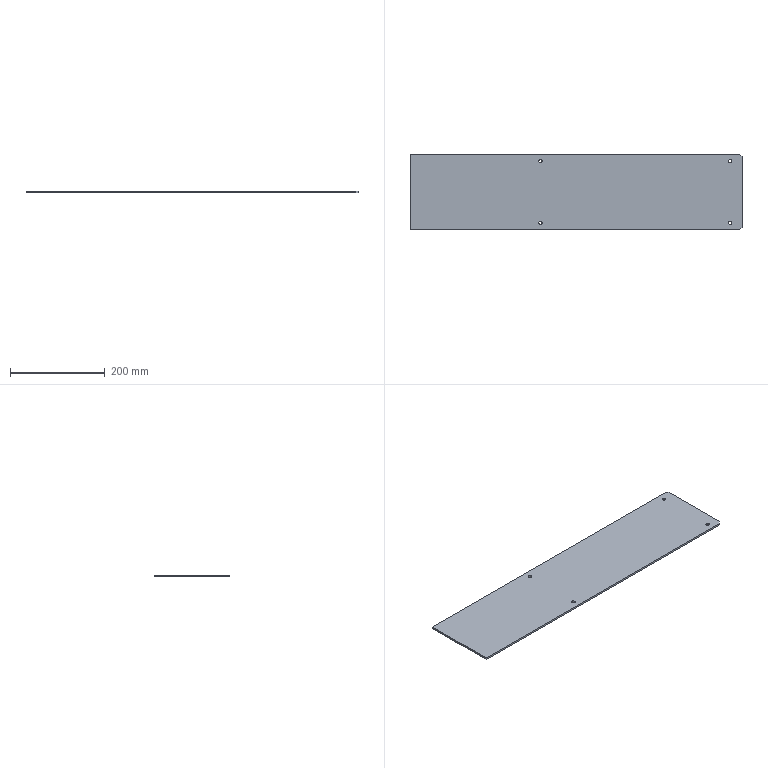Part | SolidWorks | features Chamfer 1, Extrusion 1, ICE 1 | 1 solid | 16 faces | box 700 x 160 x 4 mm | volume 447284 mm3 | cylinder 8 | plane 8 | commonest cylinder face diameters 7 x8
STEP:
#1=CARTESIAN_POINT('',(-78.5,-65.,0.));
#2=VERTEX_POINT('',#1);
#3=CARTESIAN_POINT('',(-71.5,-65.,0.));
#4=VERTEX_POINT('',#3);
#5=CARTESIAN_POINT('',(-75.,-65.,0.));
#6=DIRECTION('',(0.,0.,1.));
#7=DIRECTION('',(1.,0.,0.));
#8=AXIS2_PLACEMENT_3D('',#5,#6,#7);
#9=CIRCLE('',#8,3.5);
#10=EDGE_CURVE('',#2,#4,#9,.T.);
#11=ORIENTED_EDGE('',*,*,#10,.F.);
#12=CARTESIAN_POINT('',(-78.5,-65.,4.));
#13=VERTEX_POINT('',#12);
#14=CARTESIAN_POINT('',(-78.5,-65.,0.));
#15=DIRECTION('',(0.,0.,1.));
#16=VECTOR('',#15,1000.);
#17=LINE('',#14,#16);
#18=EDGE_CURVE('',#2,#13,#17,.T.);
#19=ORIENTED_EDGE('',*,*,#18,.T.);
#20=CARTESIAN_POINT('',(-71.5,-65.,4.));
#21=VERTEX_POINT('',#20);
#22=CARTESIAN_POINT('',(-75.,-65.,4.));
#23=DIRECTION('',(0.,0.,1.));
#24=DIRECTION('',(1.,0.,0.));
#25=AXIS2_PLACEMENT_3D('',#22,#23,#24);
#26=CIRCLE('',#25,3.5);
#27=EDGE_CURVE('',#13,#21,#26,.T.);
#28=ORIENTED_EDGE('',*,*,#27,.T.);
#29=CARTESIAN_POINT('',(-71.5,-65.,0.));
#30=DIRECTION('',(0.,0.,1.));
#31=VECTOR('',#30,1000.);
#32=LINE('',#29,#31);
#33=EDGE_CURVE('',#4,#21,#32,.T.);
#34=ORIENTED_EDGE('',*,*,#33,.F.);
#35=EDGE_LOOP('',(#11,#19,#28,#34));
#36=FACE_OUTER_BOUND('',#35,.T.);
#37=CARTESIAN_POINT('',(-75.,-65.,0.));
#38=DIRECTION('',(0.,0.,1.));
#39=DIRECTION('',(1.,0.,0.));
#40=AXIS2_PLACEMENT_3D('',#37,#38,#39);
#41=CYLINDRICAL_SURFACE('',#40,3.5);
#42=ADVANCED_FACE('',(#36),#41,.F.);
#43=CARTESIAN_POINT('',(321.5,-65.,0.));
#44=VERTEX_POINT('',#43);
#45=CARTESIAN_POINT('',(328.5,-65.,0.));
#46=VERTEX_POINT('',#45);
#47=CARTESIAN_POINT('',(325.,-65.,0.));
#48=DIRECTION('',(0.,0.,1.));
#49=DIRECTION('',(1.,0.,0.));
#50=AXIS2_PLACEMENT_3D('',#47,#48,#49);
#51=CIRCLE('',#50,3.5);
#52=EDGE_CURVE('',#44,#46,#51,.T.);
#53=ORIENTED_EDGE('',*,*,#52,.F.);
#54=CARTESIAN_POINT('',(321.5,-65.,4.));
#55=VERTEX_POINT('',#54);
#56=CARTESIAN_POINT('',(321.5,-65.,0.));
#57=DIRECTION('',(0.,0.,1.));
#58=VECTOR('',#57,1000.);
#59=LINE('',#56,#58);
#60=EDGE_CURVE('',#44,#55,#59,.T.);
#61=ORIENTED_EDGE('',*,*,#60,.T.);
#62=CARTESIAN_POINT('',(328.5,-65.,4.));
#63=VERTEX_POINT('',#62);
#64=CARTESIAN_POINT('',(325.,-65.,4.));
#65=DIRECTION('',(0.,0.,1.));
#66=DIRECTION('',(1.,0.,0.));
#67=AXIS2_PLACEMENT_3D('',#64,#65,#66);
#68=CIRCLE('',#67,3.5);
#69=EDGE_CURVE('',#55,#63,#68,.T.);
#70=ORIENTED_EDGE('',*,*,#69,.T.);
#71=CARTESIAN_POINT('',(328.5,-65.,0.));
#72=DIRECTION('',(0.,0.,1.));
#73=VECTOR('',#72,1000.);
#74=LINE('',#71,#73);
#75=EDGE_CURVE('',#46,#63,#74,.T.);
#76=ORIENTED_EDGE('',*,*,#75,.F.);
#77=EDGE_LOOP('',(#53,#61,#70,#76));
#78=FACE_OUTER_BOUND('',#77,.T.);
#79=CARTESIAN_POINT('',(325.,-65.,0.));
#80=DIRECTION('',(0.,0.,1.));
#81=DIRECTION('',(1.,0.,0.));
#82=AXIS2_PLACEMENT_3D('',#79,#80,#81);
#83=CYLINDRICAL_SURFACE('',#82,3.5);
#84=ADVANCED_FACE('',(#78),#83,.F.);
#85=CARTESIAN_POINT('',(321.5,65.,0.));
#86=VERTEX_POINT('',#85);
#87=CARTESIAN_POINT('',(328.5,65.,0.));
#88=VERTEX_POINT('',#87);
#89=CARTESIAN_POINT('',(325.,65.,0.));
#90=DIRECTION('',(0.,0.,1.));
#91=DIRECTION('',(1.,0.,0.));
#92=AXIS2_PLACEMENT_3D('',#89,#90,#91);
#93=CIRCLE('',#92,3.5);
#94=EDGE_CURVE('',#86,#88,#93,.T.);
#95=ORIENTED_EDGE('',*,*,#94,.F.);
#96=CARTESIAN_POINT('',(321.5,65.,4.));
#97=VERTEX_POINT('',#96);
#98=CARTESIAN_POINT('',(321.5,65.,0.));
#99=DIRECTION('',(0.,0.,1.));
#100=VECTOR('',#99,1000.);
#101=LINE('',#98,#100);
#102=EDGE_CURVE('',#86,#97,#101,.T.);
#103=ORIENTED_EDGE('',*,*,#102,.T.);
#104=CARTESIAN_POINT('',(328.5,65.,4.));
#105=VERTEX_POINT('',#104);
#106=CARTESIAN_POINT('',(325.,65.,4.));
#107=DIRECTION('',(0.,0.,1.));
#108=DIRECTION('',(1.,0.,0.));
#109=AXIS2_PLACEMENT_3D('',#106,#107,#108);
#110=CIRCLE('',#109,3.5);
#111=EDGE_CURVE('',#97,#105,#110,.T.);
#112=ORIENTED_EDGE('',*,*,#111,.T.);
#113=CARTESIAN_POINT('',(328.5,65.,0.));
#114=DIRECTION('',(0.,0.,1.));
#115=VECTOR('',#114,1000.);
#116=LINE('',#113,#115);
#117=EDGE_CURVE('',#88,#105,#116,.T.);
#118=ORIENTED_EDGE('',*,*,#117,.F.);
#119=EDGE_LOOP('',(#95,#103,#112,#118));
#120=FACE_OUTER_BOUND('',#119,.T.);
#121=CARTESIAN_POINT('',(325.,65.,0.));
#122=DIRECTION('',(0.,0.,1.));
#123=DIRECTION('',(1.,0.,0.));
#124=AXIS2_PLACEMENT_3D('',#121,#122,#123);
#125=CYLINDRICAL_SURFACE('',#124,3.5);
#126=ADVANCED_FACE('',(#120),#125,.F.);
#127=CARTESIAN_POINT('',(-78.5,65.,0.));
#128=VERTEX_POINT('',#127);
#129=CARTESIAN_POINT('',(-71.5,65.,0.));
#130=VERTEX_POINT('',#129);
#131=CARTESIAN_POINT('',(-75.,65.,0.));
#132=DIRECTION('',(0.,0.,1.));
#133=DIRECTION('',(1.,0.,0.));
#134=AXIS2_PLACEMENT_3D('',#131,#132,#133);
#135=CIRCLE('',#134,3.5);
#136=EDGE_CURVE('',#128,#130,#135,.T.);
#137=ORIENTED_EDGE('',*,*,#136,.F.);
#138=CARTESIAN_POINT('',(-78.5,65.,4.));
#139=VERTEX_POINT('',#138);
#140=CARTESIAN_POINT('',(-78.5,65.,0.));
#141=DIRECTION('',(0.,0.,1.));
#142=VECTOR('',#141,1000.);
#143=LINE('',#140,#142);
#144=EDGE_CURVE('',#128,#139,#143,.T.);
#145=ORIENTED_EDGE('',*,*,#144,.T.);
#146=CARTESIAN_POINT('',(-71.5,65.,4.));
#147=VERTEX_POINT('',#146);
#148=CARTESIAN_POINT('',(-75.,65.,4.));
#149=DIRECTION('',(0.,0.,1.));
#150=DIRECTION('',(1.,0.,0.));
#151=AXIS2_PLACEMENT_3D('',#148,#149,#150);
#152=CIRCLE('',#151,3.5);
#153=EDGE_CURVE('',#139,#147,#152,.T.);
#154=ORIENTED_EDGE('',*,*,#153,.T.);
#155=CARTESIAN_POINT('',(-71.5,65.,0.));
#156=DIRECTION('',(0.,0.,1.));
#157=VECTOR('',#156,1000.);
#158=LINE('',#155,#157);
#159=EDGE_CURVE('',#130,#147,#158,.T.);
#160=ORIENTED_EDGE('',*,*,#159,.F.);
#161=EDGE_LOOP('',(#137,#145,#154,#160));
#162=FACE_OUTER_BOUND('',#161,.T.);
#163=CARTESIAN_POINT('',(-75.,65.,0.));
#164=DIRECTION('',(0.,0.,1.));
#165=DIRECTION('',(1.,0.,0.));
#166=AXIS2_PLACEMENT_3D('',#163,#164,#165);
#167=CYLINDRICAL_SURFACE('',#166,3.5);
#168=ADVANCED_FACE('',(#162),#167,.F.);
#169=CARTESIAN_POINT('',(-350.,-80.,0.));
#170=VERTEX_POINT('',#169);
#171=CARTESIAN_POINT('',(345.,-80.,0.));
#172=VERTEX_POINT('',#171);
#173=CARTESIAN_POINT('',(-350.,-80.,0.));
#174=DIRECTION('',(1.,0.,0.));
#175=VECTOR('',#174,1000.);
#176=LINE('',#173,#175);
#177=EDGE_CURVE('',#170,#172,#176,.T.);
#178=ORIENTED_EDGE('',*,*,#177,.T.);
#179=CARTESIAN_POINT('',(345.,-80.,4.));
#180=VERTEX_POINT('',#179);
#181=CARTESIAN_POINT('',(345.,-80.,4.));
#182=DIRECTION('',(0.,0.,1.));
#183=VECTOR('',#182,1000.);
#184=LINE('',#181,#183);
#185=EDGE_CURVE('',#172,#180,#184,.T.);
#186=ORIENTED_EDGE('',*,*,#185,.T.);
#187=CARTESIAN_POINT('',(-350.,-80.,4.));
#188=VERTEX_POINT('',#187);
#189=CARTESIAN_POINT('',(-350.,-80.,4.));
#190=DIRECTION('',(1.,0.,0.));
#191=VECTOR('',#190,1000.);
#192=LINE('',#189,#191);
#193=EDGE_CURVE('',#188,#180,#192,.T.);
#194=ORIENTED_EDGE('',*,*,#193,.F.);
#195=CARTESIAN_POINT('',(-350.,-80.,4.));
#196=DIRECTION('',(0.,0.,-1.));
#197=VECTOR('',#196,1000.);
#198=LINE('',#195,#197);
#199=EDGE_CURVE('',#188,#170,#198,.T.);
#200=ORIENTED_EDGE('',*,*,#199,.T.);
#201=EDGE_LOOP('',(#178,#186,#194,#200));
#202=FACE_OUTER_BOUND('',#201,.T.);
#203=CARTESIAN_POINT('',(-350.,-80.,4.));
#204=DIRECTION('',(0.,1.,0.));
#205=DIRECTION('',(0.,0.,1.));
#206=AXIS2_PLACEMENT_3D('',#203,#204,#205);
#207=PLANE('',#206);
#208=ADVANCED_FACE('',(#202),#207,.F.);
#209=CARTESIAN_POINT('',(350.,75.,4.));
#210=VERTEX_POINT('',#209);
#211=CARTESIAN_POINT('',(350.,-75.,4.));
#212=VERTEX_POINT('',#211);
#213=CARTESIAN_POINT('',(350.,80.,4.));
#214=DIRECTION('',(0.,-1.,0.));
#215=VECTOR('',#214,1000.);
#216=LINE('',#213,#215);
#217=EDGE_CURVE('',#210,#212,#216,.T.);
#218=ORIENTED_EDGE('',*,*,#217,.T.);
#219=CARTESIAN_POINT('',(350.,-75.,0.));
#220=VERTEX_POINT('',#219);
#221=CARTESIAN_POINT('',(350.,-75.,0.));
#222=DIRECTION('',(0.,0.,-1.));
#223=VECTOR('',#222,1000.);
#224=LINE('',#221,#223);
#225=EDGE_CURVE('',#212,#220,#224,.T.);
#226=ORIENTED_EDGE('',*,*,#225,.T.);
#227=CARTESIAN_POINT('',(350.,75.,0.));
#228=VERTEX_POINT('',#227);
#229=CARTESIAN_POINT('',(350.,80.,0.));
#230=DIRECTION('',(0.,-1.,0.));
#231=VECTOR('',#230,1000.);
#232=LINE('',#229,#231);
#233=EDGE_CURVE('',#228,#220,#232,.T.);
#234=ORIENTED_EDGE('',*,*,#233,.F.);
#235=CARTESIAN_POINT('',(350.,75.,4.));
#236=DIRECTION('',(0.,0.,1.));
#237=VECTOR('',#236,1000.);
#238=LINE('',#235,#237);
#239=EDGE_CURVE('',#228,#210,#238,.T.);
#240=ORIENTED_EDGE('',*,*,#239,.T.);
#241=EDGE_LOOP('',(#218,#226,#234,#240));
#242=FACE_OUTER_BOUND('',#241,.T.);
#243=CARTESIAN_POINT('',(350.,80.,4.));
#244=DIRECTION('',(1.,0.,0.));
#245=DIRECTION('',(0.,0.,-1.));
#246=AXIS2_PLACEMENT_3D('',#243,#244,#245);
#247=PLANE('',#246);
#248=ADVANCED_FACE('',(#242),#247,.T.);
#249=CARTESIAN_POINT('',(-350.,80.,4.));
#250=VERTEX_POINT('',#249);
#251=CARTESIAN_POINT('',(345.,80.,4.));
#252=VERTEX_POINT('',#251);
#253=CARTESIAN_POINT('',(-350.,80.,4.));
#254=DIRECTION('',(1.,0.,0.));
#255=VECTOR('',#254,1000.);
#256=LINE('',#253,#255);
#257=EDGE_CURVE('',#250,#252,#256,.T.);
#258=ORIENTED_EDGE('',*,*,#257,.T.);
#259=CARTESIAN_POINT('',(345.,80.,0.));
#260=VERTEX_POINT('',#259);
#261=CARTESIAN_POINT('',(345.,80.,4.));
#262=DIRECTION('',(0.,0.,-1.));
#263=VECTOR('',#262,1000.);
#264=LINE('',#261,#263);
#265=EDGE_CURVE('',#252,#260,#264,.T.);
#266=ORIENTED_EDGE('',*,*,#265,.T.);
#267=CARTESIAN_POINT('',(-350.,80.,0.));
#268=VERTEX_POINT('',#267);
#269=CARTESIAN_POINT('',(-350.,80.,0.));
#270=DIRECTION('',(1.,0.,0.));
#271=VECTOR('',#270,1000.);
#272=LINE('',#269,#271);
#273=EDGE_CURVE('',#268,#260,#272,.T.);
#274=ORIENTED_EDGE('',*,*,#273,.F.);
#275=CARTESIAN_POINT('',(-350.,80.,4.));
#276=DIRECTION('',(0.,0.,-1.));
#277=VECTOR('',#276,1000.);
#278=LINE('',#275,#277);
#279=EDGE_CURVE('',#250,#268,#278,.T.);
#280=ORIENTED_EDGE('',*,*,#279,.F.);
#281=EDGE_LOOP('',(#258,#266,#274,#280));
#282=FACE_OUTER_BOUND('',#281,.T.);
#283=CARTESIAN_POINT('',(-350.,80.,4.));
#284=DIRECTION('',(0.,1.,0.));
#285=DIRECTION('',(0.,0.,1.));
#286=AXIS2_PLACEMENT_3D('',#283,#284,#285);
#287=PLANE('',#286);
#288=ADVANCED_FACE('',(#282),#287,.T.);
#289=CARTESIAN_POINT('',(-350.,80.,0.));
#290=DIRECTION('',(0.,-1.,0.));
#291=VECTOR('',#290,1000.);
#292=LINE('',#289,#291);
#293=EDGE_CURVE('',#268,#170,#292,.T.);
#294=ORIENTED_EDGE('',*,*,#293,.T.);
#295=ORIENTED_EDGE('',*,*,#199,.F.);
#296=CARTESIAN_POINT('',(-350.,80.,4.));
#297=DIRECTION('',(0.,-1.,0.));
#298=VECTOR('',#297,1000.);
#299=LINE('',#296,#298);
#300=EDGE_CURVE('',#250,#188,#299,.T.);
#301=ORIENTED_EDGE('',*,*,#300,.F.);
#302=ORIENTED_EDGE('',*,*,#279,.T.);
#303=EDGE_LOOP('',(#294,#295,#301,#302));
#304=FACE_OUTER_BOUND('',#303,.T.);
#305=CARTESIAN_POINT('',(-350.,80.,4.));
#306=DIRECTION('',(1.,0.,0.));
#307=DIRECTION('',(0.,1.,0.));
#308=AXIS2_PLACEMENT_3D('',#305,#306,#307);
#309=PLANE('',#308);
#310=ADVANCED_FACE('',(#304),#309,.F.);
#311=CARTESIAN_POINT('',(-75.,-65.,4.));
#312=DIRECTION('',(0.,0.,1.));
#313=DIRECTION('',(1.,0.,0.));
#314=AXIS2_PLACEMENT_3D('',#311,#312,#313);
#315=CIRCLE('',#314,3.5);
#316=EDGE_CURVE('',#21,#13,#315,.T.);
#317=ORIENTED_EDGE('',*,*,#316,.F.);
#318=ORIENTED_EDGE('',*,*,#27,.F.);
#319=EDGE_LOOP('',(#317,#318));
#320=FACE_BOUND('',#319,.T.);
#321=CARTESIAN_POINT('',(325.,-65.,4.));
#322=DIRECTION('',(0.,0.,1.));
#323=DIRECTION('',(1.,0.,0.));
#324=AXIS2_PLACEMENT_3D('',#321,#322,#323);
#325=CIRCLE('',#324,3.5);
#326=EDGE_CURVE('',#63,#55,#325,.T.);
#327=ORIENTED_EDGE('',*,*,#326,.F.);
#328=ORIENTED_EDGE('',*,*,#69,.F.);
#329=EDGE_LOOP('',(#327,#328));
#330=FACE_BOUND('',#329,.T.);
#331=CARTESIAN_POINT('',(325.,65.,4.));
#332=DIRECTION('',(0.,0.,1.));
#333=DIRECTION('',(1.,0.,0.));
#334=AXIS2_PLACEMENT_3D('',#331,#332,#333);
#335=CIRCLE('',#334,3.5);
#336=EDGE_CURVE('',#105,#97,#335,.T.);
#337=ORIENTED_EDGE('',*,*,#336,.F.);
#338=ORIENTED_EDGE('',*,*,#111,.F.);
#339=EDGE_LOOP('',(#337,#338));
#340=FACE_BOUND('',#339,.T.);
#341=CARTESIAN_POINT('',(-75.,65.,4.));
#342=DIRECTION('',(0.,0.,1.));
#343=DIRECTION('',(1.,0.,0.));
#344=AXIS2_PLACEMENT_3D('',#341,#342,#343);
#345=CIRCLE('',#344,3.5);
#346=EDGE_CURVE('',#147,#139,#345,.T.);
#347=ORIENTED_EDGE('',*,*,#346,.F.);
#348=ORIENTED_EDGE('',*,*,#153,.F.);
#349=EDGE_LOOP('',(#347,#348));
#350=FACE_BOUND('',#349,.T.);
#351=ORIENTED_EDGE('',*,*,#193,.T.);
#352=CARTESIAN_POINT('',(350.,-75.,4.));
#353=DIRECTION('',(0.7071,0.7071,0.));
#354=VECTOR('',#353,1000.);
#355=LINE('',#352,#354);
#356=EDGE_CURVE('',#180,#212,#355,.T.);
#357=ORIENTED_EDGE('',*,*,#356,.T.);
#358=ORIENTED_EDGE('',*,*,#217,.F.);
#359=CARTESIAN_POINT('',(345.,80.,4.));
#360=DIRECTION('',(-0.7071,0.7071,0.));
#361=VECTOR('',#360,1000.);
#362=LINE('',#359,#361);
#363=EDGE_CURVE('',#210,#252,#362,.T.);
#364=ORIENTED_EDGE('',*,*,#363,.T.);
#365=ORIENTED_EDGE('',*,*,#257,.F.);
#366=ORIENTED_EDGE('',*,*,#300,.T.);
#367=EDGE_LOOP('',(#351,#357,#358,#364,#365,#366));
#368=FACE_OUTER_BOUND('',#367,.T.);
#369=CARTESIAN_POINT('',(0.,0.,4.));
#370=DIRECTION('',(0.,0.,-1.));
#371=DIRECTION('',(-1.,0.,0.));
#372=AXIS2_PLACEMENT_3D('',#369,#370,#371);
#373=PLANE('',#372);
#374=ADVANCED_FACE('',(#320,#330,#340,#350,#368),#373,.F.);
#375=CARTESIAN_POINT('',(-75.,-65.,0.));
#376=DIRECTION('',(0.,0.,1.));
#377=DIRECTION('',(1.,0.,0.));
#378=AXIS2_PLACEMENT_3D('',#375,#376,#377);
#379=CIRCLE('',#378,3.5);
#380=EDGE_CURVE('',#4,#2,#379,.T.);
#381=ORIENTED_EDGE('',*,*,#380,.T.);
#382=ORIENTED_EDGE('',*,*,#10,.T.);
#383=EDGE_LOOP('',(#381,#382));
#384=FACE_BOUND('',#383,.T.);
#385=CARTESIAN_POINT('',(325.,-65.,0.));
#386=DIRECTION('',(0.,0.,1.));
#387=DIRECTION('',(1.,0.,0.));
#388=AXIS2_PLACEMENT_3D('',#385,#386,#387);
#389=CIRCLE('',#388,3.5);
#390=EDGE_CURVE('',#46,#44,#389,.T.);
#391=ORIENTED_EDGE('',*,*,#390,.T.);
#392=ORIENTED_EDGE('',*,*,#52,.T.);
#393=EDGE_LOOP('',(#391,#392));
#394=FACE_BOUND('',#393,.T.);
#395=CARTESIAN_POINT('',(325.,65.,0.));
#396=DIRECTION('',(0.,0.,1.));
#397=DIRECTION('',(1.,0.,0.));
#398=AXIS2_PLACEMENT_3D('',#395,#396,#397);
#399=CIRCLE('',#398,3.5);
#400=EDGE_CURVE('',#88,#86,#399,.T.);
#401=ORIENTED_EDGE('',*,*,#400,.T.);
#402=ORIENTED_EDGE('',*,*,#94,.T.);
#403=EDGE_LOOP('',(#401,#402));
#404=FACE_BOUND('',#403,.T.);
#405=CARTESIAN_POINT('',(-75.,65.,0.));
#406=DIRECTION('',(0.,0.,1.));
#407=DIRECTION('',(1.,0.,0.));
#408=AXIS2_PLACEMENT_3D('',#405,#406,#407);
#409=CIRCLE('',#408,3.5);
#410=EDGE_CURVE('',#130,#128,#409,.T.);
#411=ORIENTED_EDGE('',*,*,#410,.T.);
#412=ORIENTED_EDGE('',*,*,#136,.T.);
#413=EDGE_LOOP('',(#411,#412));
#414=FACE_BOUND('',#413,.T.);
#415=ORIENTED_EDGE('',*,*,#233,.T.);
#416=CARTESIAN_POINT('',(212.5,-212.5,0.));
#417=DIRECTION('',(-0.7071,-0.7071,0.));
#418=VECTOR('',#417,1000.);
#419=LINE('',#416,#418);
#420=EDGE_CURVE('',#220,#172,#419,.T.);
#421=ORIENTED_EDGE('',*,*,#420,.T.);
#422=ORIENTED_EDGE('',*,*,#177,.F.);
#423=ORIENTED_EDGE('',*,*,#293,.F.);
#424=ORIENTED_EDGE('',*,*,#273,.T.);
#425=CARTESIAN_POINT('',(212.5,212.5,0.));
#426=DIRECTION('',(0.7071,-0.7071,0.));
#427=VECTOR('',#426,1000.);
#428=LINE('',#425,#427);
#429=EDGE_CURVE('',#260,#228,#428,.T.);
#430=ORIENTED_EDGE('',*,*,#429,.T.);
#431=EDGE_LOOP('',(#415,#421,#422,#423,#424,#430));
#432=FACE_OUTER_BOUND('',#431,.T.);
#433=CARTESIAN_POINT('',(0.,0.,0.));
#434=DIRECTION('',(0.,0.,-1.));
#435=DIRECTION('',(-1.,0.,0.));
#436=AXIS2_PLACEMENT_3D('',#433,#434,#435);
#437=PLANE('',#436);
#438=ADVANCED_FACE('',(#384,#394,#404,#414,#432),#437,.T.);
#439=ORIENTED_EDGE('',*,*,#144,.F.);
#440=ORIENTED_EDGE('',*,*,#410,.F.);
#441=ORIENTED_EDGE('',*,*,#159,.T.);
#442=ORIENTED_EDGE('',*,*,#346,.T.);
#443=EDGE_LOOP('',(#439,#440,#441,#442));
#444=FACE_OUTER_BOUND('',#443,.T.);
#445=CARTESIAN_POINT('',(-75.,65.,0.));
#446=DIRECTION('',(0.,0.,1.));
#447=DIRECTION('',(1.,0.,0.));
#448=AXIS2_PLACEMENT_3D('',#445,#446,#447);
#449=CYLINDRICAL_SURFACE('',#448,3.5);
#450=ADVANCED_FACE('',(#444),#449,.F.);
#451=ORIENTED_EDGE('',*,*,#102,.F.);
#452=ORIENTED_EDGE('',*,*,#400,.F.);
#453=ORIENTED_EDGE('',*,*,#117,.T.);
#454=ORIENTED_EDGE('',*,*,#336,.T.);
#455=EDGE_LOOP('',(#451,#452,#453,#454));
#456=FACE_OUTER_BOUND('',#455,.T.);
#457=CARTESIAN_POINT('',(325.,65.,0.));
#458=DIRECTION('',(0.,0.,1.));
#459=DIRECTION('',(1.,0.,0.));
#460=AXIS2_PLACEMENT_3D('',#457,#458,#459);
#461=CYLINDRICAL_SURFACE('',#460,3.5);
#462=ADVANCED_FACE('',(#456),#461,.F.);
#463=ORIENTED_EDGE('',*,*,#60,.F.);
#464=ORIENTED_EDGE('',*,*,#390,.F.);
#465=ORIENTED_EDGE('',*,*,#75,.T.);
#466=ORIENTED_EDGE('',*,*,#326,.T.);
#467=EDGE_LOOP('',(#463,#464,#465,#466));
#468=FACE_OUTER_BOUND('',#467,.T.);
#469=CARTESIAN_POINT('',(325.,-65.,0.));
#470=DIRECTION('',(0.,0.,1.));
#471=DIRECTION('',(1.,0.,0.));
#472=AXIS2_PLACEMENT_3D('',#469,#470,#471);
#473=CYLINDRICAL_SURFACE('',#472,3.5);
#474=ADVANCED_FACE('',(#468),#473,.F.);
#475=ORIENTED_EDGE('',*,*,#18,.F.);
#476=ORIENTED_EDGE('',*,*,#380,.F.);
#477=ORIENTED_EDGE('',*,*,#33,.T.);
#478=ORIENTED_EDGE('',*,*,#316,.T.);
#479=EDGE_LOOP('',(#475,#476,#477,#478));
#480=FACE_OUTER_BOUND('',#479,.T.);
#481=CARTESIAN_POINT('',(-75.,-65.,0.));
#482=DIRECTION('',(0.,0.,1.));
#483=DIRECTION('',(1.,0.,0.));
#484=AXIS2_PLACEMENT_3D('',#481,#482,#483);
#485=CYLINDRICAL_SURFACE('',#484,3.5);
#486=ADVANCED_FACE('',(#480),#485,.F.);
#487=ORIENTED_EDGE('',*,*,#356,.F.);
#488=ORIENTED_EDGE('',*,*,#185,.F.);
#489=ORIENTED_EDGE('',*,*,#420,.F.);
#490=ORIENTED_EDGE('',*,*,#225,.F.);
#491=EDGE_LOOP('',(#487,#488,#489,#490));
#492=FACE_OUTER_BOUND('',#491,.T.);
#493=CARTESIAN_POINT('',(350.,-75.,4.));
#494=DIRECTION('',(0.7071,-0.7071,0.));
#495=DIRECTION('',(0.,0.,1.));
#496=AXIS2_PLACEMENT_3D('',#493,#494,#495);
#497=PLANE('',#496);
#498=ADVANCED_FACE('',(#492),#497,.T.);
#499=ORIENTED_EDGE('',*,*,#363,.F.);
#500=ORIENTED_EDGE('',*,*,#239,.F.);
#501=ORIENTED_EDGE('',*,*,#429,.F.);
#502=ORIENTED_EDGE('',*,*,#265,.F.);
#503=EDGE_LOOP('',(#499,#500,#501,#502));
#504=FACE_OUTER_BOUND('',#503,.T.);
#505=CARTESIAN_POINT('',(345.,80.,4.));
#506=DIRECTION('',(-0.7071,-0.7071,0.));
#507=DIRECTION('',(0.,0.,-1.));
#508=AXIS2_PLACEMENT_3D('',#505,#506,#507);
#509=PLANE('',#508);
#510=ADVANCED_FACE('',(#504),#509,.F.);
#511=CLOSED_SHELL('',(#42,#84,#126,#168,#208,#248,#288,#310,#374,#438,#450,#462,#474,#486,#498,#510));
#512=MANIFOLD_SOLID_BREP('',#511);
#513=CARTESIAN_POINT('',(0.,0.,0.));
#514=DIRECTION('',(0.,0.,1.));
#515=DIRECTION('',(1.,0.,0.));
#516=AXIS2_PLACEMENT_3D('',#513,#514,#515);
#517=(LENGTH_UNIT()NAMED_UNIT(*)SI_UNIT(.MILLI.,.METRE.));
#518=UNCERTAINTY_MEASURE_WITH_UNIT(LENGTH_MEASURE(0.00001),#517,'','');
#519=(NAMED_UNIT(*)PLANE_ANGLE_UNIT()SI_UNIT($,.RADIAN.));
#520=(NAMED_UNIT(*)SI_UNIT($,.STERADIAN.)SOLID_ANGLE_UNIT());
#521=(GEOMETRIC_REPRESENTATION_CONTEXT(3)GLOBAL_UNCERTAINTY_ASSIGNED_CONTEXT((#518))GLOBAL_UNIT_ASSIGNED_CONTEXT((#517,#519,#520))REPRESENTATION_CONTEXT('',''));
#522=ADVANCED_BREP_SHAPE_REPRESENTATION('',(#512,#516),#521);